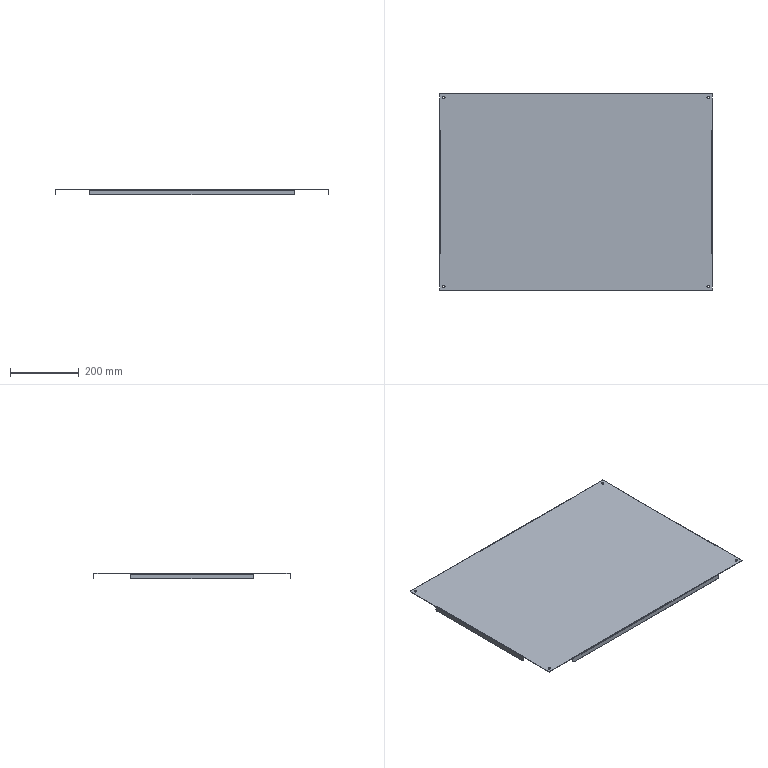Part | SolidWorks | features BaseBody 1 | 1 solid | 90 faces | box 795 x 575 x 15 mm | volume 579015 mm3 | plane 62 | cylinder 28 | commonest cylinder face diameters 7 x8 10 x8 1 x4 3.4 x4 4 x4